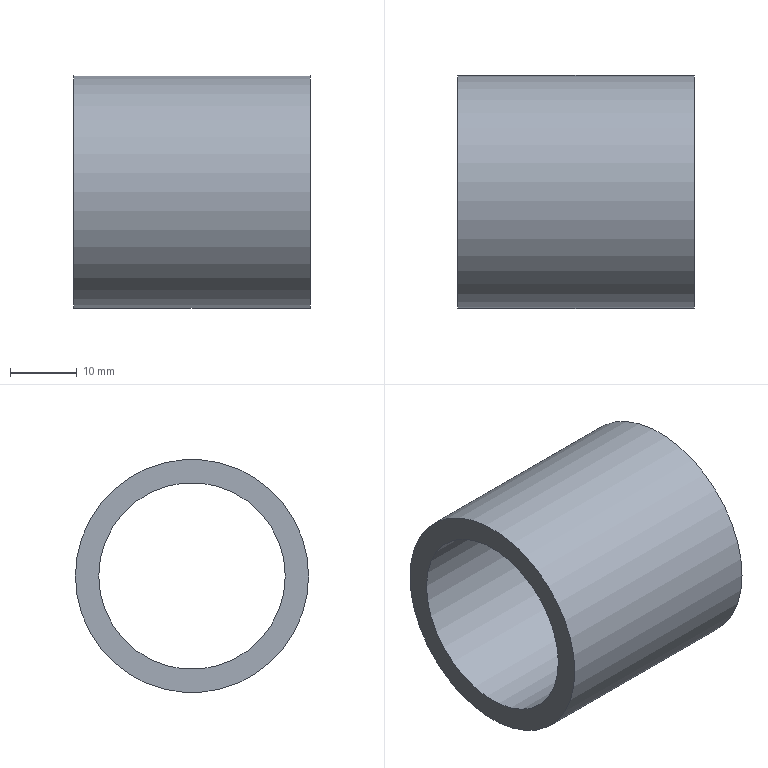Part | NX | features DATUM_CSYS 2, EXTRUDE 1, SKETCH 1 | 1 solid | 4 faces | box 35.5 x 35 x 35 mm | volume 12296 mm3 | cylinder 2 | plane 2 | commonest cylinder face diameters 28 x1 35 x1
STEP:
#1=CARTESIAN_POINT('',(35.5,17.5,0.));
#2=VERTEX_POINT('',#1);
#3=CARTESIAN_POINT('',(35.5,0.,0.));
#4=DIRECTION('',(1.,0.,0.));
#5=DIRECTION('',(0.,1.,0.));
#6=AXIS2_PLACEMENT_3D('',#3,#4,#5);
#7=CIRCLE('',#6,17.5);
#8=EDGE_CURVE('',#2,#2,#7,.T.);
#9=ORIENTED_EDGE('',*,*,#8,.F.);
#10=EDGE_LOOP('',(#9));
#11=FACE_BOUND('',#10,.T.);
#12=CARTESIAN_POINT('',(0.,17.5,0.));
#13=VERTEX_POINT('',#12);
#14=CARTESIAN_POINT('',(0.,0.,0.));
#15=DIRECTION('',(1.,0.,0.));
#16=DIRECTION('',(0.,1.,0.));
#17=AXIS2_PLACEMENT_3D('',#14,#15,#16);
#18=CIRCLE('',#17,17.5);
#19=EDGE_CURVE('',#13,#13,#18,.T.);
#20=ORIENTED_EDGE('',*,*,#19,.T.);
#21=EDGE_LOOP('',(#20));
#22=FACE_BOUND('',#21,.T.);
#23=CARTESIAN_POINT('',(35.5,0.,0.));
#24=DIRECTION('',(-1.,0.,0.));
#25=DIRECTION('',(0.,0.,1.));
#26=AXIS2_PLACEMENT_3D('',#23,#24,#25);
#27=CYLINDRICAL_SURFACE('',#26,17.5);
#28=ADVANCED_FACE('',(#11,#22),#27,.T.);
#29=CARTESIAN_POINT('',(35.5,14.,0.));
#30=VERTEX_POINT('',#29);
#31=CARTESIAN_POINT('',(35.5,0.,0.));
#32=DIRECTION('',(1.,0.,0.));
#33=DIRECTION('',(0.,1.,0.));
#34=AXIS2_PLACEMENT_3D('',#31,#32,#33);
#35=CIRCLE('',#34,14.);
#36=EDGE_CURVE('',#30,#30,#35,.T.);
#37=ORIENTED_EDGE('',*,*,#36,.T.);
#38=EDGE_LOOP('',(#37));
#39=FACE_BOUND('',#38,.T.);
#40=CARTESIAN_POINT('',(0.,14.,0.));
#41=VERTEX_POINT('',#40);
#42=CARTESIAN_POINT('',(0.,0.,0.));
#43=DIRECTION('',(1.,0.,0.));
#44=DIRECTION('',(0.,1.,0.));
#45=AXIS2_PLACEMENT_3D('',#42,#43,#44);
#46=CIRCLE('',#45,14.);
#47=EDGE_CURVE('',#41,#41,#46,.T.);
#48=ORIENTED_EDGE('',*,*,#47,.F.);
#49=EDGE_LOOP('',(#48));
#50=FACE_BOUND('',#49,.T.);
#51=CARTESIAN_POINT('',(35.5,0.,0.));
#52=DIRECTION('',(-1.,0.,0.));
#53=DIRECTION('',(0.,0.,1.));
#54=AXIS2_PLACEMENT_3D('',#51,#52,#53);
#55=CYLINDRICAL_SURFACE('',#54,14.);
#56=ADVANCED_FACE('',(#39,#50),#55,.F.);
#57=ORIENTED_EDGE('',*,*,#8,.T.);
#58=EDGE_LOOP('',(#57));
#59=FACE_BOUND('',#58,.T.);
#60=ORIENTED_EDGE('',*,*,#36,.F.);
#61=EDGE_LOOP('',(#60));
#62=FACE_BOUND('',#61,.T.);
#63=CARTESIAN_POINT('',(35.5,0.,0.));
#64=DIRECTION('',(1.,0.,0.));
#65=DIRECTION('',(0.,0.,-1.));
#66=AXIS2_PLACEMENT_3D('',#63,#64,#65);
#67=PLANE('',#66);
#68=ADVANCED_FACE('',(#59,#62),#67,.T.);
#69=ORIENTED_EDGE('',*,*,#19,.F.);
#70=EDGE_LOOP('',(#69));
#71=FACE_BOUND('',#70,.T.);
#72=ORIENTED_EDGE('',*,*,#47,.T.);
#73=EDGE_LOOP('',(#72));
#74=FACE_BOUND('',#73,.T.);
#75=CARTESIAN_POINT('',(0.,0.,0.));
#76=DIRECTION('',(1.,0.,0.));
#77=DIRECTION('',(0.,0.,-1.));
#78=AXIS2_PLACEMENT_3D('',#75,#76,#77);
#79=PLANE('',#78);
#80=ADVANCED_FACE('',(#71,#74),#79,.F.);
#81=CLOSED_SHELL('',(#28,#56,#68,#80));
#82=MANIFOLD_SOLID_BREP('',#81);
#83=(LENGTH_UNIT()NAMED_UNIT(*)SI_UNIT(.MILLI.,.METRE.));
#84=UNCERTAINTY_MEASURE_WITH_UNIT(LENGTH_MEASURE(0.00001),#83,'','');
#85=(NAMED_UNIT(*)PLANE_ANGLE_UNIT()SI_UNIT($,.RADIAN.));
#86=(NAMED_UNIT(*)SI_UNIT($,.STERADIAN.)SOLID_ANGLE_UNIT());
#87=(GEOMETRIC_REPRESENTATION_CONTEXT(3)GLOBAL_UNCERTAINTY_ASSIGNED_CONTEXT((#84))GLOBAL_UNIT_ASSIGNED_CONTEXT((#83,#85,#86))REPRESENTATION_CONTEXT('',''));
#88=ADVANCED_BREP_SHAPE_REPRESENTATION('',(#82),#87);